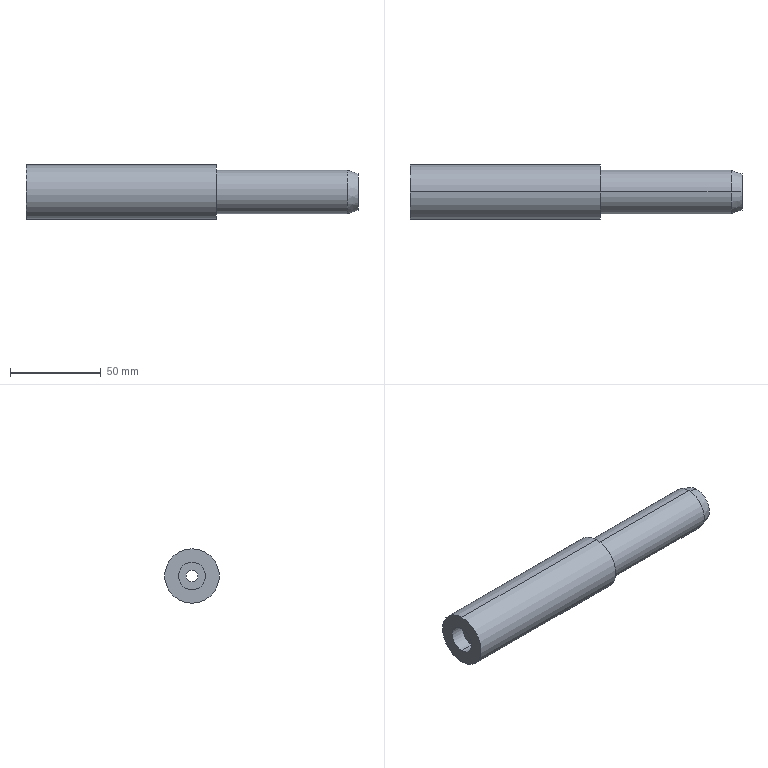Part | SolidWorks | features Chamfer 1, Revolution 1 | 1 solid | 17 faces | box 183 x 30 x 30 mm | volume 80329 mm3 | cylinder 10 | plane 5 | cone 2 | commonest cylinder face diameters 15 x4 6.5 x2 24 x2 30 x2
STEP:
#1=CARTESIAN_POINT('',(183.,0.,-10.));
#2=VERTEX_POINT('',#1);
#3=CARTESIAN_POINT('',(183.,0.,10.));
#4=VERTEX_POINT('',#3);
#5=CARTESIAN_POINT('',(183.,0.,0.));
#6=DIRECTION('',(1.,0.,0.));
#7=DIRECTION('',(0.,0.,1.));
#8=AXIS2_PLACEMENT_3D('',#5,#6,#7);
#9=CIRCLE('',#8,10.);
#10=EDGE_CURVE('',#2,#4,#9,.T.);
#11=ORIENTED_EDGE('',*,*,#10,.F.);
#12=CARTESIAN_POINT('',(177.,0.,-12.));
#13=VERTEX_POINT('',#12);
#14=CARTESIAN_POINT('',(177.,0.,-12.));
#15=DIRECTION('',(-0.9487,0.,-0.3162));
#16=VECTOR('',#15,1000.);
#17=LINE('',#14,#16);
#18=EDGE_CURVE('',#2,#13,#17,.T.);
#19=ORIENTED_EDGE('',*,*,#18,.T.);
#20=CARTESIAN_POINT('',(177.,0.,12.));
#21=VERTEX_POINT('',#20);
#22=CARTESIAN_POINT('',(177.,0.,0.));
#23=DIRECTION('',(-1.,0.,0.));
#24=DIRECTION('',(0.,0.,1.));
#25=AXIS2_PLACEMENT_3D('',#22,#23,#24);
#26=CIRCLE('',#25,12.);
#27=EDGE_CURVE('',#21,#13,#26,.T.);
#28=ORIENTED_EDGE('',*,*,#27,.F.);
#29=CARTESIAN_POINT('',(177.,0.,12.));
#30=DIRECTION('',(-0.9487,0.,0.3162));
#31=VECTOR('',#30,1000.);
#32=LINE('',#29,#31);
#33=EDGE_CURVE('',#4,#21,#32,.T.);
#34=ORIENTED_EDGE('',*,*,#33,.F.);
#35=EDGE_LOOP('',(#11,#19,#28,#34));
#36=FACE_OUTER_BOUND('',#35,.T.);
#37=CARTESIAN_POINT('',(177.,0.,0.));
#38=DIRECTION('',(-1.,0.,0.));
#39=DIRECTION('',(0.,0.,1.));
#40=AXIS2_PLACEMENT_3D('',#37,#38,#39);
#41=CONICAL_SURFACE('',#40,12.,0.3218);
#42=ADVANCED_FACE('',(#36),#41,.T.);
#43=CARTESIAN_POINT('',(33.,0.,-3.25));
#44=VERTEX_POINT('',#43);
#45=CARTESIAN_POINT('',(33.,0.,3.25));
#46=VERTEX_POINT('',#45);
#47=CARTESIAN_POINT('',(33.,0.,0.));
#48=DIRECTION('',(-1.,0.,0.));
#49=DIRECTION('',(0.,0.,1.));
#50=AXIS2_PLACEMENT_3D('',#47,#48,#49);
#51=CIRCLE('',#50,3.25);
#52=EDGE_CURVE('',#44,#46,#51,.T.);
#53=ORIENTED_EDGE('',*,*,#52,.F.);
#54=CARTESIAN_POINT('',(8.,0.,-3.25));
#55=VERTEX_POINT('',#54);
#56=CARTESIAN_POINT('',(0.,0.,-3.25));
#57=DIRECTION('',(-1.,0.,0.));
#58=VECTOR('',#57,1000.);
#59=LINE('',#56,#58);
#60=EDGE_CURVE('',#44,#55,#59,.T.);
#61=ORIENTED_EDGE('',*,*,#60,.T.);
#62=CARTESIAN_POINT('',(8.,0.,3.25));
#63=VERTEX_POINT('',#62);
#64=CARTESIAN_POINT('',(8.,0.,0.));
#65=DIRECTION('',(-1.,0.,0.));
#66=DIRECTION('',(0.,0.,1.));
#67=AXIS2_PLACEMENT_3D('',#64,#65,#66);
#68=CIRCLE('',#67,3.25);
#69=EDGE_CURVE('',#55,#63,#68,.T.);
#70=ORIENTED_EDGE('',*,*,#69,.T.);
#71=CARTESIAN_POINT('',(0.,0.,3.25));
#72=DIRECTION('',(-1.,0.,0.));
#73=VECTOR('',#72,1000.);
#74=LINE('',#71,#73);
#75=EDGE_CURVE('',#46,#63,#74,.T.);
#76=ORIENTED_EDGE('',*,*,#75,.F.);
#77=EDGE_LOOP('',(#53,#61,#70,#76));
#78=FACE_OUTER_BOUND('',#77,.T.);
#79=CARTESIAN_POINT('',(0.,0.,0.));
#80=DIRECTION('',(-1.,0.,0.));
#81=DIRECTION('',(0.,0.,1.));
#82=AXIS2_PLACEMENT_3D('',#79,#80,#81);
#83=CYLINDRICAL_SURFACE('',#82,3.25);
#84=ADVANCED_FACE('',(#78),#83,.F.);
#85=CARTESIAN_POINT('',(183.,0.,-7.5));
#86=VERTEX_POINT('',#85);
#87=CARTESIAN_POINT('',(183.,0.,7.5));
#88=VERTEX_POINT('',#87);
#89=CARTESIAN_POINT('',(183.,0.,0.));
#90=DIRECTION('',(-1.,0.,0.));
#91=DIRECTION('',(0.,0.,1.));
#92=AXIS2_PLACEMENT_3D('',#89,#90,#91);
#93=CIRCLE('',#92,7.5);
#94=EDGE_CURVE('',#86,#88,#93,.T.);
#95=ORIENTED_EDGE('',*,*,#94,.F.);
#96=CARTESIAN_POINT('',(33.,0.,-7.5));
#97=VERTEX_POINT('',#96);
#98=CARTESIAN_POINT('',(0.,0.,-7.5));
#99=DIRECTION('',(-1.,0.,0.));
#100=VECTOR('',#99,1000.);
#101=LINE('',#98,#100);
#102=EDGE_CURVE('',#86,#97,#101,.T.);
#103=ORIENTED_EDGE('',*,*,#102,.T.);
#104=CARTESIAN_POINT('',(33.,0.,7.5));
#105=VERTEX_POINT('',#104);
#106=CARTESIAN_POINT('',(33.,0.,0.));
#107=DIRECTION('',(-1.,0.,0.));
#108=DIRECTION('',(0.,0.,1.));
#109=AXIS2_PLACEMENT_3D('',#106,#107,#108);
#110=CIRCLE('',#109,7.5);
#111=EDGE_CURVE('',#97,#105,#110,.T.);
#112=ORIENTED_EDGE('',*,*,#111,.T.);
#113=CARTESIAN_POINT('',(0.,0.,7.5));
#114=DIRECTION('',(-1.,0.,0.));
#115=VECTOR('',#114,1000.);
#116=LINE('',#113,#115);
#117=EDGE_CURVE('',#88,#105,#116,.T.);
#118=ORIENTED_EDGE('',*,*,#117,.F.);
#119=EDGE_LOOP('',(#95,#103,#112,#118));
#120=FACE_OUTER_BOUND('',#119,.T.);
#121=CARTESIAN_POINT('',(0.,0.,0.));
#122=DIRECTION('',(-1.,0.,0.));
#123=DIRECTION('',(0.,0.,1.));
#124=AXIS2_PLACEMENT_3D('',#121,#122,#123);
#125=CYLINDRICAL_SURFACE('',#124,7.5);
#126=ADVANCED_FACE('',(#120),#125,.F.);
#127=ORIENTED_EDGE('',*,*,#27,.T.);
#128=CARTESIAN_POINT('',(105.,0.,-12.));
#129=VERTEX_POINT('',#128);
#130=CARTESIAN_POINT('',(0.,0.,-12.));
#131=DIRECTION('',(-1.,0.,0.));
#132=VECTOR('',#131,1000.);
#133=LINE('',#130,#132);
#134=EDGE_CURVE('',#13,#129,#133,.T.);
#135=ORIENTED_EDGE('',*,*,#134,.T.);
#136=CARTESIAN_POINT('',(105.,0.,12.));
#137=VERTEX_POINT('',#136);
#138=CARTESIAN_POINT('',(105.,0.,0.));
#139=DIRECTION('',(-1.,0.,0.));
#140=DIRECTION('',(0.,0.,1.));
#141=AXIS2_PLACEMENT_3D('',#138,#139,#140);
#142=CIRCLE('',#141,12.);
#143=EDGE_CURVE('',#137,#129,#142,.T.);
#144=ORIENTED_EDGE('',*,*,#143,.F.);
#145=CARTESIAN_POINT('',(0.,0.,12.));
#146=DIRECTION('',(-1.,0.,0.));
#147=VECTOR('',#146,1000.);
#148=LINE('',#145,#147);
#149=EDGE_CURVE('',#21,#137,#148,.T.);
#150=ORIENTED_EDGE('',*,*,#149,.F.);
#151=EDGE_LOOP('',(#127,#135,#144,#150));
#152=FACE_OUTER_BOUND('',#151,.T.);
#153=CARTESIAN_POINT('',(0.,0.,0.));
#154=DIRECTION('',(-1.,0.,0.));
#155=DIRECTION('',(0.,0.,1.));
#156=AXIS2_PLACEMENT_3D('',#153,#154,#155);
#157=CYLINDRICAL_SURFACE('',#156,12.);
#158=ADVANCED_FACE('',(#152),#157,.T.);
#159=CARTESIAN_POINT('',(105.,0.,15.));
#160=VERTEX_POINT('',#159);
#161=CARTESIAN_POINT('',(105.,0.,-15.));
#162=VERTEX_POINT('',#161);
#163=CARTESIAN_POINT('',(105.,0.,0.));
#164=DIRECTION('',(-1.,0.,0.));
#165=DIRECTION('',(0.,0.,1.));
#166=AXIS2_PLACEMENT_3D('',#163,#164,#165);
#167=CIRCLE('',#166,15.);
#168=EDGE_CURVE('',#160,#162,#167,.T.);
#169=ORIENTED_EDGE('',*,*,#168,.T.);
#170=CARTESIAN_POINT('',(0.,0.,-15.));
#171=VERTEX_POINT('',#170);
#172=CARTESIAN_POINT('',(0.,0.,-15.));
#173=DIRECTION('',(-1.,0.,0.));
#174=VECTOR('',#173,1000.);
#175=LINE('',#172,#174);
#176=EDGE_CURVE('',#162,#171,#175,.T.);
#177=ORIENTED_EDGE('',*,*,#176,.T.);
#178=CARTESIAN_POINT('',(0.,0.,15.));
#179=VERTEX_POINT('',#178);
#180=CARTESIAN_POINT('',(0.,0.,0.));
#181=DIRECTION('',(-1.,0.,0.));
#182=DIRECTION('',(0.,0.,1.));
#183=AXIS2_PLACEMENT_3D('',#180,#181,#182);
#184=CIRCLE('',#183,15.);
#185=EDGE_CURVE('',#179,#171,#184,.T.);
#186=ORIENTED_EDGE('',*,*,#185,.F.);
#187=CARTESIAN_POINT('',(0.,0.,15.));
#188=DIRECTION('',(-1.,0.,0.));
#189=VECTOR('',#188,1000.);
#190=LINE('',#187,#189);
#191=EDGE_CURVE('',#160,#179,#190,.T.);
#192=ORIENTED_EDGE('',*,*,#191,.F.);
#193=EDGE_LOOP('',(#169,#177,#186,#192));
#194=FACE_OUTER_BOUND('',#193,.T.);
#195=CARTESIAN_POINT('',(0.,0.,0.));
#196=DIRECTION('',(-1.,0.,0.));
#197=DIRECTION('',(0.,0.,1.));
#198=AXIS2_PLACEMENT_3D('',#195,#196,#197);
#199=CYLINDRICAL_SURFACE('',#198,15.);
#200=ADVANCED_FACE('',(#194),#199,.T.);
#201=CARTESIAN_POINT('',(8.,0.,-7.5));
#202=VERTEX_POINT('',#201);
#203=CARTESIAN_POINT('',(8.,0.,7.5));
#204=VERTEX_POINT('',#203);
#205=CARTESIAN_POINT('',(8.,0.,0.));
#206=DIRECTION('',(-1.,0.,0.));
#207=DIRECTION('',(0.,0.,1.));
#208=AXIS2_PLACEMENT_3D('',#205,#206,#207);
#209=CIRCLE('',#208,7.5);
#210=EDGE_CURVE('',#202,#204,#209,.T.);
#211=ORIENTED_EDGE('',*,*,#210,.F.);
#212=CARTESIAN_POINT('',(0.,0.,-7.5));
#213=VERTEX_POINT('',#212);
#214=CARTESIAN_POINT('',(0.,0.,-7.5));
#215=DIRECTION('',(-1.,0.,0.));
#216=VECTOR('',#215,1000.);
#217=LINE('',#214,#216);
#218=EDGE_CURVE('',#202,#213,#217,.T.);
#219=ORIENTED_EDGE('',*,*,#218,.T.);
#220=CARTESIAN_POINT('',(0.,0.,7.5));
#221=VERTEX_POINT('',#220);
#222=CARTESIAN_POINT('',(0.,0.,0.));
#223=DIRECTION('',(-1.,0.,0.));
#224=DIRECTION('',(0.,0.,1.));
#225=AXIS2_PLACEMENT_3D('',#222,#223,#224);
#226=CIRCLE('',#225,7.5);
#227=EDGE_CURVE('',#213,#221,#226,.T.);
#228=ORIENTED_EDGE('',*,*,#227,.T.);
#229=CARTESIAN_POINT('',(0.,0.,7.5));
#230=DIRECTION('',(-1.,0.,0.));
#231=VECTOR('',#230,1000.);
#232=LINE('',#229,#231);
#233=EDGE_CURVE('',#204,#221,#232,.T.);
#234=ORIENTED_EDGE('',*,*,#233,.F.);
#235=EDGE_LOOP('',(#211,#219,#228,#234));
#236=FACE_OUTER_BOUND('',#235,.T.);
#237=CARTESIAN_POINT('',(0.,0.,0.));
#238=DIRECTION('',(-1.,0.,0.));
#239=DIRECTION('',(0.,0.,1.));
#240=AXIS2_PLACEMENT_3D('',#237,#238,#239);
#241=CYLINDRICAL_SURFACE('',#240,7.5);
#242=ADVANCED_FACE('',(#236),#241,.F.);
#243=ORIENTED_EDGE('',*,*,#218,.F.);
#244=CARTESIAN_POINT('',(8.,0.,0.));
#245=DIRECTION('',(-1.,0.,0.));
#246=DIRECTION('',(0.,0.,1.));
#247=AXIS2_PLACEMENT_3D('',#244,#245,#246);
#248=CIRCLE('',#247,7.5);
#249=EDGE_CURVE('',#204,#202,#248,.T.);
#250=ORIENTED_EDGE('',*,*,#249,.F.);
#251=ORIENTED_EDGE('',*,*,#233,.T.);
#252=CARTESIAN_POINT('',(0.,0.,0.));
#253=DIRECTION('',(-1.,0.,0.));
#254=DIRECTION('',(0.,0.,1.));
#255=AXIS2_PLACEMENT_3D('',#252,#253,#254);
#256=CIRCLE('',#255,7.5);
#257=EDGE_CURVE('',#221,#213,#256,.T.);
#258=ORIENTED_EDGE('',*,*,#257,.T.);
#259=EDGE_LOOP('',(#243,#250,#251,#258));
#260=FACE_OUTER_BOUND('',#259,.T.);
#261=CARTESIAN_POINT('',(0.,0.,0.));
#262=DIRECTION('',(-1.,0.,0.));
#263=DIRECTION('',(0.,0.,1.));
#264=AXIS2_PLACEMENT_3D('',#261,#262,#263);
#265=CYLINDRICAL_SURFACE('',#264,7.5);
#266=ADVANCED_FACE('',(#260),#265,.F.);
#267=ORIENTED_EDGE('',*,*,#257,.F.);
#268=ORIENTED_EDGE('',*,*,#227,.F.);
#269=EDGE_LOOP('',(#267,#268));
#270=FACE_BOUND('',#269,.T.);
#271=ORIENTED_EDGE('',*,*,#185,.T.);
#272=CARTESIAN_POINT('',(0.,0.,0.));
#273=DIRECTION('',(-1.,0.,0.));
#274=DIRECTION('',(0.,0.,1.));
#275=AXIS2_PLACEMENT_3D('',#272,#273,#274);
#276=CIRCLE('',#275,15.);
#277=EDGE_CURVE('',#171,#179,#276,.T.);
#278=ORIENTED_EDGE('',*,*,#277,.T.);
#279=EDGE_LOOP('',(#271,#278));
#280=FACE_OUTER_BOUND('',#279,.T.);
#281=CARTESIAN_POINT('',(0.,7.5,0.));
#282=DIRECTION('',(1.,0.,0.));
#283=DIRECTION('',(0.,0.,-1.));
#284=AXIS2_PLACEMENT_3D('',#281,#282,#283);
#285=PLANE('',#284);
#286=ADVANCED_FACE('',(#270,#280),#285,.F.);
#287=ORIENTED_EDGE('',*,*,#176,.F.);
#288=CARTESIAN_POINT('',(105.,0.,0.));
#289=DIRECTION('',(-1.,0.,0.));
#290=DIRECTION('',(0.,0.,1.));
#291=AXIS2_PLACEMENT_3D('',#288,#289,#290);
#292=CIRCLE('',#291,15.);
#293=EDGE_CURVE('',#162,#160,#292,.T.);
#294=ORIENTED_EDGE('',*,*,#293,.T.);
#295=ORIENTED_EDGE('',*,*,#191,.T.);
#296=ORIENTED_EDGE('',*,*,#277,.F.);
#297=EDGE_LOOP('',(#287,#294,#295,#296));
#298=FACE_OUTER_BOUND('',#297,.T.);
#299=CARTESIAN_POINT('',(0.,0.,0.));
#300=DIRECTION('',(-1.,0.,0.));
#301=DIRECTION('',(0.,0.,1.));
#302=AXIS2_PLACEMENT_3D('',#299,#300,#301);
#303=CYLINDRICAL_SURFACE('',#302,15.);
#304=ADVANCED_FACE('',(#298),#303,.T.);
#305=ORIENTED_EDGE('',*,*,#168,.F.);
#306=ORIENTED_EDGE('',*,*,#293,.F.);
#307=EDGE_LOOP('',(#305,#306));
#308=FACE_OUTER_BOUND('',#307,.T.);
#309=ORIENTED_EDGE('',*,*,#143,.T.);
#310=CARTESIAN_POINT('',(105.,0.,0.));
#311=DIRECTION('',(-1.,0.,0.));
#312=DIRECTION('',(0.,0.,1.));
#313=AXIS2_PLACEMENT_3D('',#310,#311,#312);
#314=CIRCLE('',#313,12.);
#315=EDGE_CURVE('',#129,#137,#314,.T.);
#316=ORIENTED_EDGE('',*,*,#315,.T.);
#317=EDGE_LOOP('',(#309,#316));
#318=FACE_BOUND('',#317,.T.);
#319=CARTESIAN_POINT('',(105.,12.,0.));
#320=DIRECTION('',(-1.,0.,0.));
#321=DIRECTION('',(0.,0.,1.));
#322=AXIS2_PLACEMENT_3D('',#319,#320,#321);
#323=PLANE('',#322);
#324=ADVANCED_FACE('',(#308,#318),#323,.F.);
#325=ORIENTED_EDGE('',*,*,#134,.F.);
#326=CARTESIAN_POINT('',(177.,0.,0.));
#327=DIRECTION('',(-1.,0.,0.));
#328=DIRECTION('',(0.,0.,1.));
#329=AXIS2_PLACEMENT_3D('',#326,#327,#328);
#330=CIRCLE('',#329,12.);
#331=EDGE_CURVE('',#13,#21,#330,.T.);
#332=ORIENTED_EDGE('',*,*,#331,.T.);
#333=ORIENTED_EDGE('',*,*,#149,.T.);
#334=ORIENTED_EDGE('',*,*,#315,.F.);
#335=EDGE_LOOP('',(#325,#332,#333,#334));
#336=FACE_OUTER_BOUND('',#335,.T.);
#337=CARTESIAN_POINT('',(0.,0.,0.));
#338=DIRECTION('',(-1.,0.,0.));
#339=DIRECTION('',(0.,0.,1.));
#340=AXIS2_PLACEMENT_3D('',#337,#338,#339);
#341=CYLINDRICAL_SURFACE('',#340,12.);
#342=ADVANCED_FACE('',(#336),#341,.T.);
#343=CARTESIAN_POINT('',(183.,0.,0.));
#344=DIRECTION('',(1.,0.,0.));
#345=DIRECTION('',(0.,0.,1.));
#346=AXIS2_PLACEMENT_3D('',#343,#344,#345);
#347=CIRCLE('',#346,10.);
#348=EDGE_CURVE('',#4,#2,#347,.T.);
#349=ORIENTED_EDGE('',*,*,#348,.T.);
#350=ORIENTED_EDGE('',*,*,#10,.T.);
#351=EDGE_LOOP('',(#349,#350));
#352=FACE_OUTER_BOUND('',#351,.T.);
#353=CARTESIAN_POINT('',(183.,0.,0.));
#354=DIRECTION('',(-1.,0.,0.));
#355=DIRECTION('',(0.,0.,1.));
#356=AXIS2_PLACEMENT_3D('',#353,#354,#355);
#357=CIRCLE('',#356,7.5);
#358=EDGE_CURVE('',#88,#86,#357,.T.);
#359=ORIENTED_EDGE('',*,*,#358,.T.);
#360=ORIENTED_EDGE('',*,*,#94,.T.);
#361=EDGE_LOOP('',(#359,#360));
#362=FACE_BOUND('',#361,.T.);
#363=CARTESIAN_POINT('',(183.,12.,0.));
#364=DIRECTION('',(-1.,0.,0.));
#365=DIRECTION('',(0.,0.,1.));
#366=AXIS2_PLACEMENT_3D('',#363,#364,#365);
#367=PLANE('',#366);
#368=ADVANCED_FACE('',(#352,#362),#367,.F.);
#369=ORIENTED_EDGE('',*,*,#102,.F.);
#370=ORIENTED_EDGE('',*,*,#358,.F.);
#371=ORIENTED_EDGE('',*,*,#117,.T.);
#372=CARTESIAN_POINT('',(33.,0.,0.));
#373=DIRECTION('',(-1.,0.,0.));
#374=DIRECTION('',(0.,0.,1.));
#375=AXIS2_PLACEMENT_3D('',#372,#373,#374);
#376=CIRCLE('',#375,7.5);
#377=EDGE_CURVE('',#105,#97,#376,.T.);
#378=ORIENTED_EDGE('',*,*,#377,.T.);
#379=EDGE_LOOP('',(#369,#370,#371,#378));
#380=FACE_OUTER_BOUND('',#379,.T.);
#381=CARTESIAN_POINT('',(0.,0.,0.));
#382=DIRECTION('',(-1.,0.,0.));
#383=DIRECTION('',(0.,0.,1.));
#384=AXIS2_PLACEMENT_3D('',#381,#382,#383);
#385=CYLINDRICAL_SURFACE('',#384,7.5);
#386=ADVANCED_FACE('',(#380),#385,.F.);
#387=ORIENTED_EDGE('',*,*,#377,.F.);
#388=ORIENTED_EDGE('',*,*,#111,.F.);
#389=EDGE_LOOP('',(#387,#388));
#390=FACE_OUTER_BOUND('',#389,.T.);
#391=CARTESIAN_POINT('',(33.,0.,0.));
#392=DIRECTION('',(-1.,0.,0.));
#393=DIRECTION('',(0.,0.,1.));
#394=AXIS2_PLACEMENT_3D('',#391,#392,#393);
#395=CIRCLE('',#394,3.25);
#396=EDGE_CURVE('',#46,#44,#395,.T.);
#397=ORIENTED_EDGE('',*,*,#396,.T.);
#398=ORIENTED_EDGE('',*,*,#52,.T.);
#399=EDGE_LOOP('',(#397,#398));
#400=FACE_BOUND('',#399,.T.);
#401=CARTESIAN_POINT('',(33.,3.25,0.));
#402=DIRECTION('',(-1.,0.,0.));
#403=DIRECTION('',(0.,0.,1.));
#404=AXIS2_PLACEMENT_3D('',#401,#402,#403);
#405=PLANE('',#404);
#406=ADVANCED_FACE('',(#390,#400),#405,.F.);
#407=ORIENTED_EDGE('',*,*,#60,.F.);
#408=ORIENTED_EDGE('',*,*,#396,.F.);
#409=ORIENTED_EDGE('',*,*,#75,.T.);
#410=CARTESIAN_POINT('',(8.,0.,0.));
#411=DIRECTION('',(-1.,0.,0.));
#412=DIRECTION('',(0.,0.,1.));
#413=AXIS2_PLACEMENT_3D('',#410,#411,#412);
#414=CIRCLE('',#413,3.25);
#415=EDGE_CURVE('',#63,#55,#414,.T.);
#416=ORIENTED_EDGE('',*,*,#415,.T.);
#417=EDGE_LOOP('',(#407,#408,#409,#416));
#418=FACE_OUTER_BOUND('',#417,.T.);
#419=CARTESIAN_POINT('',(0.,0.,0.));
#420=DIRECTION('',(-1.,0.,0.));
#421=DIRECTION('',(0.,0.,1.));
#422=AXIS2_PLACEMENT_3D('',#419,#420,#421);
#423=CYLINDRICAL_SURFACE('',#422,3.25);
#424=ADVANCED_FACE('',(#418),#423,.F.);
#425=ORIENTED_EDGE('',*,*,#415,.F.);
#426=ORIENTED_EDGE('',*,*,#69,.F.);
#427=EDGE_LOOP('',(#425,#426));
#428=FACE_BOUND('',#427,.T.);
#429=ORIENTED_EDGE('',*,*,#249,.T.);
#430=ORIENTED_EDGE('',*,*,#210,.T.);
#431=EDGE_LOOP('',(#429,#430));
#432=FACE_OUTER_BOUND('',#431,.T.);
#433=CARTESIAN_POINT('',(8.,7.5,0.));
#434=DIRECTION('',(1.,0.,0.));
#435=DIRECTION('',(0.,0.,-1.));
#436=AXIS2_PLACEMENT_3D('',#433,#434,#435);
#437=PLANE('',#436);
#438=ADVANCED_FACE('',(#428,#432),#437,.F.);
#439=ORIENTED_EDGE('',*,*,#18,.F.);
#440=ORIENTED_EDGE('',*,*,#348,.F.);
#441=ORIENTED_EDGE('',*,*,#33,.T.);
#442=ORIENTED_EDGE('',*,*,#331,.F.);
#443=EDGE_LOOP('',(#439,#440,#441,#442));
#444=FACE_OUTER_BOUND('',#443,.T.);
#445=CARTESIAN_POINT('',(177.,0.,0.));
#446=DIRECTION('',(-1.,0.,0.));
#447=DIRECTION('',(0.,0.,1.));
#448=AXIS2_PLACEMENT_3D('',#445,#446,#447);
#449=CONICAL_SURFACE('',#448,12.,0.3218);
#450=ADVANCED_FACE('',(#444),#449,.T.);
#451=CLOSED_SHELL('',(#42,#84,#126,#158,#200,#242,#266,#286,#304,#324,#342,#368,#386,#406,#424,#438,#450));
#452=MANIFOLD_SOLID_BREP('',#451);
#453=CARTESIAN_POINT('',(0.,0.,0.));
#454=DIRECTION('',(0.,0.,1.));
#455=DIRECTION('',(1.,0.,0.));
#456=AXIS2_PLACEMENT_3D('',#453,#454,#455);
#457=(LENGTH_UNIT()NAMED_UNIT(*)SI_UNIT(.MILLI.,.METRE.));
#458=UNCERTAINTY_MEASURE_WITH_UNIT(LENGTH_MEASURE(0.00001),#457,'','');
#459=(NAMED_UNIT(*)PLANE_ANGLE_UNIT()SI_UNIT($,.RADIAN.));
#460=(NAMED_UNIT(*)SI_UNIT($,.STERADIAN.)SOLID_ANGLE_UNIT());
#461=(GEOMETRIC_REPRESENTATION_CONTEXT(3)GLOBAL_UNCERTAINTY_ASSIGNED_CONTEXT((#458))GLOBAL_UNIT_ASSIGNED_CONTEXT((#457,#459,#460))REPRESENTATION_CONTEXT('',''));
#462=ADVANCED_BREP_SHAPE_REPRESENTATION('',(#452,#456),#461);